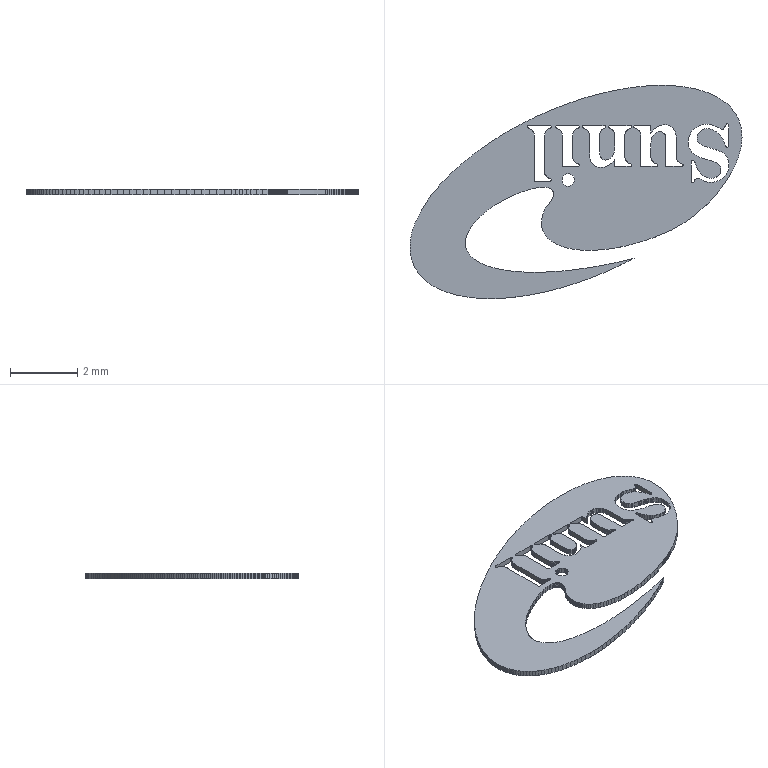Part | STEP file | LABEL-B.1A.stp | 1 solid | 1129 faces | box 9.877 x 6.344 x 0.16 mm | volume 5.062 mm3 | plane 1128 | cylinder 1 | commonest cylinder face diameters 7.556 x1